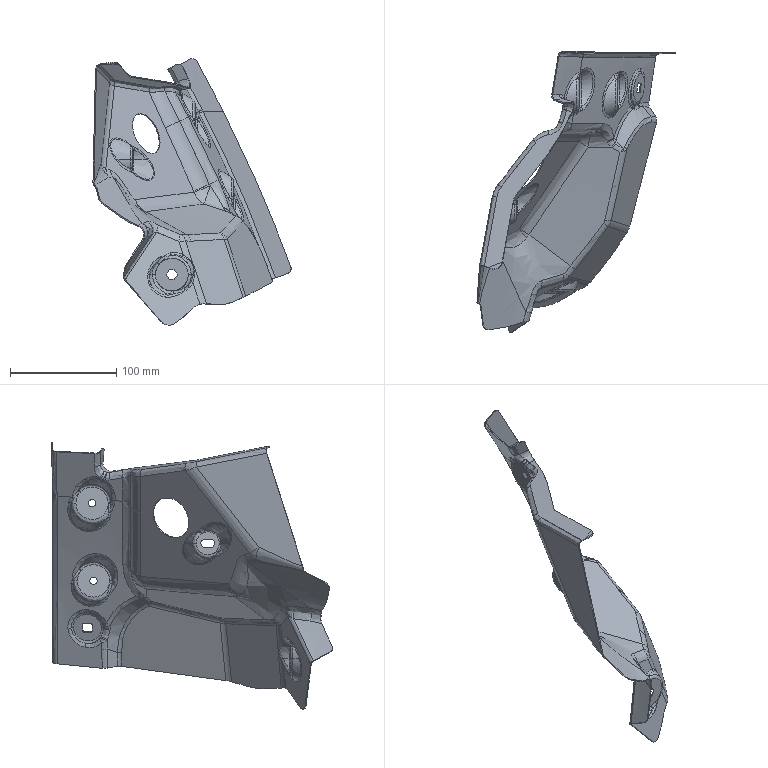Part | STEP file | FNA5401431 | 1 solid | 411 faces | box 186.295 x 264.478 x 250.717 mm | volume 73850 mm3 | spline 335 | plane 34 | cylinder 33 | sphere 6 | other 3 | commonest cylinder face diameters 2 x10 7 x4 40 x3 8 x2 10 x2 12 x1